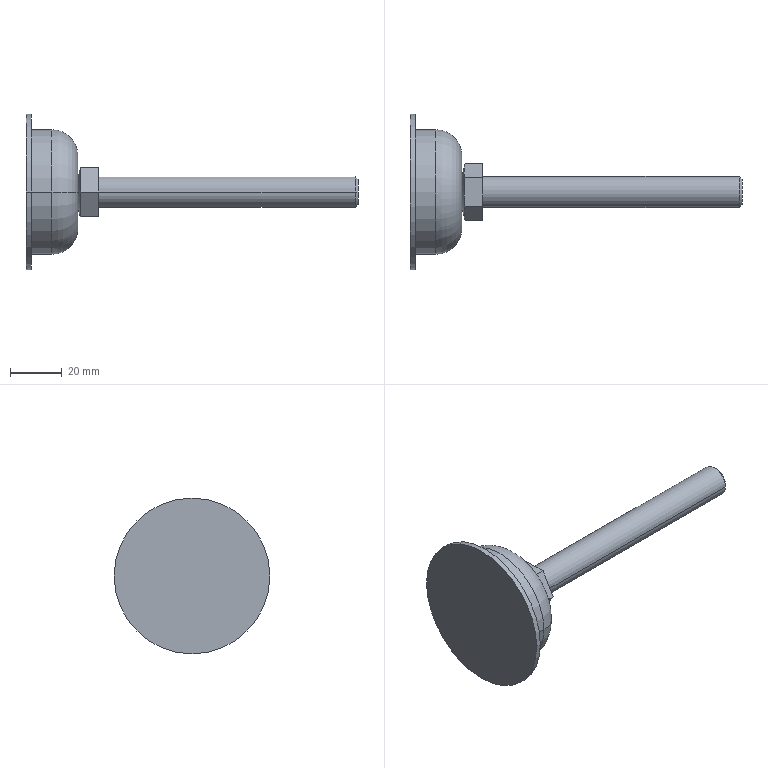Part | SolidWorks | features RefAxis 9, 3DProfileFeature 3, ICE 1, Revolution 1 | 1 solid | 23 faces | box 128 x 60 x 60 mm | volume 48974 mm3 | plane 11 | cylinder 6 | cone 4 | torus 2 | commonest cylinder face diameters 12 x2 48 x2 60 x2
STEP:
#1=CARTESIAN_POINT('',(28.,6.,0.));
#2=VERTEX_POINT('',#1);
#3=CARTESIAN_POINT('',(28.,-6.,0.));
#4=VERTEX_POINT('',#3);
#5=CARTESIAN_POINT('',(28.,0.,0.));
#6=DIRECTION('',(1.,0.,0.));
#7=DIRECTION('',(0.,1.,0.));
#8=AXIS2_PLACEMENT_3D('',#5,#6,#7);
#9=CIRCLE('',#8,6.);
#10=EDGE_CURVE('',#2,#4,#9,.T.);
#11=ORIENTED_EDGE('',*,*,#10,.T.);
#12=CARTESIAN_POINT('',(126.927,-6.,0.));
#13=VERTEX_POINT('',#12);
#14=CARTESIAN_POINT('',(0.,-6.,0.));
#15=DIRECTION('',(1.,0.,0.));
#16=VECTOR('',#15,1000.);
#17=LINE('',#14,#16);
#18=EDGE_CURVE('',#4,#13,#17,.T.);
#19=ORIENTED_EDGE('',*,*,#18,.T.);
#20=CARTESIAN_POINT('',(126.927,6.,0.));
#21=VERTEX_POINT('',#20);
#22=CARTESIAN_POINT('',(126.927,0.,0.));
#23=DIRECTION('',(1.,0.,0.));
#24=DIRECTION('',(0.,1.,0.));
#25=AXIS2_PLACEMENT_3D('',#22,#23,#24);
#26=CIRCLE('',#25,6.);
#27=EDGE_CURVE('',#21,#13,#26,.T.);
#28=ORIENTED_EDGE('',*,*,#27,.F.);
#29=CARTESIAN_POINT('',(0.,6.,0.));
#30=DIRECTION('',(1.,0.,0.));
#31=VECTOR('',#30,1000.);
#32=LINE('',#29,#31);
#33=EDGE_CURVE('',#2,#21,#32,.T.);
#34=ORIENTED_EDGE('',*,*,#33,.F.);
#35=EDGE_LOOP('',(#11,#19,#28,#34));
#36=FACE_OUTER_BOUND('',#35,.T.);
#37=CARTESIAN_POINT('',(0.,0.,0.));
#38=DIRECTION('',(1.,0.,0.));
#39=DIRECTION('',(0.,1.,0.));
#40=AXIS2_PLACEMENT_3D('',#37,#38,#39);
#41=CYLINDRICAL_SURFACE('',#40,6.);
#42=ADVANCED_FACE('',(#36),#41,.T.);
#43=CARTESIAN_POINT('',(128.,4.927,0.));
#44=VERTEX_POINT('',#43);
#45=CARTESIAN_POINT('',(128.,-4.926,0.));
#46=VERTEX_POINT('',#45);
#47=CARTESIAN_POINT('',(128.,0.,0.));
#48=DIRECTION('',(1.,0.,0.));
#49=DIRECTION('',(0.,1.,0.));
#50=AXIS2_PLACEMENT_3D('',#47,#48,#49);
#51=CIRCLE('',#50,4.926);
#52=EDGE_CURVE('',#44,#46,#51,.T.);
#53=ORIENTED_EDGE('',*,*,#52,.F.);
#54=CARTESIAN_POINT('',(126.927,6.,0.));
#55=DIRECTION('',(-0.7071,0.7071,0.));
#56=VECTOR('',#55,1000.);
#57=LINE('',#54,#56);
#58=EDGE_CURVE('',#44,#21,#57,.T.);
#59=ORIENTED_EDGE('',*,*,#58,.T.);
#60=ORIENTED_EDGE('',*,*,#27,.T.);
#61=CARTESIAN_POINT('',(126.927,-6.,0.));
#62=DIRECTION('',(-0.7071,-0.7071,0.));
#63=VECTOR('',#62,1000.);
#64=LINE('',#61,#63);
#65=EDGE_CURVE('',#46,#13,#64,.T.);
#66=ORIENTED_EDGE('',*,*,#65,.F.);
#67=EDGE_LOOP('',(#53,#59,#60,#66));
#68=FACE_OUTER_BOUND('',#67,.T.);
#69=CARTESIAN_POINT('',(126.927,0.,0.));
#70=DIRECTION('',(-1.,0.,0.));
#71=DIRECTION('',(0.,-1.,0.));
#72=AXIS2_PLACEMENT_3D('',#69,#70,#71);
#73=CONICAL_SURFACE('',#72,6.,0.7854);
#74=ADVANCED_FACE('',(#68),#73,.T.);
#75=CARTESIAN_POINT('',(0.,30.,0.));
#76=VERTEX_POINT('',#75);
#77=CARTESIAN_POINT('',(0.,-30.,0.));
#78=VERTEX_POINT('',#77);
#79=CARTESIAN_POINT('',(0.,0.,0.));
#80=DIRECTION('',(1.,0.,0.));
#81=DIRECTION('',(0.,1.,0.));
#82=AXIS2_PLACEMENT_3D('',#79,#80,#81);
#83=CIRCLE('',#82,30.);
#84=EDGE_CURVE('',#76,#78,#83,.T.);
#85=ORIENTED_EDGE('',*,*,#84,.T.);
#86=CARTESIAN_POINT('',(2.,-30.,0.));
#87=VERTEX_POINT('',#86);
#88=CARTESIAN_POINT('',(0.,-30.,0.));
#89=DIRECTION('',(1.,0.,0.));
#90=VECTOR('',#89,1000.);
#91=LINE('',#88,#90);
#92=EDGE_CURVE('',#78,#87,#91,.T.);
#93=ORIENTED_EDGE('',*,*,#92,.T.);
#94=CARTESIAN_POINT('',(2.,30.,0.));
#95=VERTEX_POINT('',#94);
#96=CARTESIAN_POINT('',(2.,0.,0.));
#97=DIRECTION('',(1.,0.,0.));
#98=DIRECTION('',(0.,1.,0.));
#99=AXIS2_PLACEMENT_3D('',#96,#97,#98);
#100=CIRCLE('',#99,30.);
#101=EDGE_CURVE('',#95,#87,#100,.T.);
#102=ORIENTED_EDGE('',*,*,#101,.F.);
#103=CARTESIAN_POINT('',(0.,30.,0.));
#104=DIRECTION('',(1.,0.,0.));
#105=VECTOR('',#104,1000.);
#106=LINE('',#103,#105);
#107=EDGE_CURVE('',#76,#95,#106,.T.);
#108=ORIENTED_EDGE('',*,*,#107,.F.);
#109=EDGE_LOOP('',(#85,#93,#102,#108));
#110=FACE_OUTER_BOUND('',#109,.T.);
#111=CARTESIAN_POINT('',(0.,0.,0.));
#112=DIRECTION('',(1.,0.,0.));
#113=DIRECTION('',(0.,1.,0.));
#114=AXIS2_PLACEMENT_3D('',#111,#112,#113);
#115=CYLINDRICAL_SURFACE('',#114,30.);
#116=ADVANCED_FACE('',(#110),#115,.T.);
#117=CARTESIAN_POINT('',(2.,24.,0.));
#118=VERTEX_POINT('',#117);
#119=CARTESIAN_POINT('',(2.,-24.,0.));
#120=VERTEX_POINT('',#119);
#121=CARTESIAN_POINT('',(2.,0.,0.));
#122=DIRECTION('',(1.,0.,0.));
#123=DIRECTION('',(0.,1.,0.));
#124=AXIS2_PLACEMENT_3D('',#121,#122,#123);
#125=CIRCLE('',#124,24.);
#126=EDGE_CURVE('',#118,#120,#125,.T.);
#127=ORIENTED_EDGE('',*,*,#126,.T.);
#128=CARTESIAN_POINT('',(10.,-24.,0.));
#129=VERTEX_POINT('',#128);
#130=CARTESIAN_POINT('',(0.,-24.,0.));
#131=DIRECTION('',(1.,0.,0.));
#132=VECTOR('',#131,1000.);
#133=LINE('',#130,#132);
#134=EDGE_CURVE('',#120,#129,#133,.T.);
#135=ORIENTED_EDGE('',*,*,#134,.T.);
#136=CARTESIAN_POINT('',(10.,24.,0.));
#137=VERTEX_POINT('',#136);
#138=CARTESIAN_POINT('',(10.,0.,0.));
#139=DIRECTION('',(1.,0.,0.));
#140=DIRECTION('',(0.,1.,0.));
#141=AXIS2_PLACEMENT_3D('',#138,#139,#140);
#142=CIRCLE('',#141,24.);
#143=EDGE_CURVE('',#137,#129,#142,.T.);
#144=ORIENTED_EDGE('',*,*,#143,.F.);
#145=CARTESIAN_POINT('',(0.,24.,0.));
#146=DIRECTION('',(1.,0.,0.));
#147=VECTOR('',#146,1000.);
#148=LINE('',#145,#147);
#149=EDGE_CURVE('',#118,#137,#148,.T.);
#150=ORIENTED_EDGE('',*,*,#149,.F.);
#151=EDGE_LOOP('',(#127,#135,#144,#150));
#152=FACE_OUTER_BOUND('',#151,.T.);
#153=CARTESIAN_POINT('',(0.,0.,0.));
#154=DIRECTION('',(1.,0.,0.));
#155=DIRECTION('',(0.,1.,0.));
#156=AXIS2_PLACEMENT_3D('',#153,#154,#155);
#157=CYLINDRICAL_SURFACE('',#156,24.);
#158=ADVANCED_FACE('',(#152),#157,.T.);
#159=ORIENTED_EDGE('',*,*,#143,.T.);
#160=CARTESIAN_POINT('',(20.,-14.,0.));
#161=VERTEX_POINT('',#160);
#162=CARTESIAN_POINT('',(10.,-14.,0.));
#163=DIRECTION('',(0.,0.,1.));
#164=DIRECTION('',(0.,-1.,0.));
#165=AXIS2_PLACEMENT_3D('',#162,#163,#164);
#166=CIRCLE('',#165,10.);
#167=EDGE_CURVE('',#129,#161,#166,.T.);
#168=ORIENTED_EDGE('',*,*,#167,.T.);
#169=CARTESIAN_POINT('',(20.,14.,0.));
#170=VERTEX_POINT('',#169);
#171=CARTESIAN_POINT('',(20.,0.,0.));
#172=DIRECTION('',(1.,0.,0.));
#173=DIRECTION('',(0.,1.,0.));
#174=AXIS2_PLACEMENT_3D('',#171,#172,#173);
#175=CIRCLE('',#174,14.);
#176=EDGE_CURVE('',#170,#161,#175,.T.);
#177=ORIENTED_EDGE('',*,*,#176,.F.);
#178=CARTESIAN_POINT('',(10.,14.,0.));
#179=DIRECTION('',(0.,0.,-1.));
#180=DIRECTION('',(-1.,0.,0.));
#181=AXIS2_PLACEMENT_3D('',#178,#179,#180);
#182=CIRCLE('',#181,10.);
#183=EDGE_CURVE('',#137,#170,#182,.T.);
#184=ORIENTED_EDGE('',*,*,#183,.F.);
#185=EDGE_LOOP('',(#159,#168,#177,#184));
#186=FACE_OUTER_BOUND('',#185,.T.);
#187=CARTESIAN_POINT('',(10.,0.,0.));
#188=DIRECTION('',(1.,0.,0.));
#189=DIRECTION('',(0.,1.,0.));
#190=AXIS2_PLACEMENT_3D('',#187,#188,#189);
#191=TOROIDAL_SURFACE('',#190,14.,10.);
#192=ADVANCED_FACE('',(#186),#191,.T.);
#193=CARTESIAN_POINT('',(20.,6.,0.));
#194=VERTEX_POINT('',#193);
#195=CARTESIAN_POINT('',(20.,-6.,0.));
#196=VERTEX_POINT('',#195);
#197=CARTESIAN_POINT('',(20.,0.,0.));
#198=DIRECTION('',(1.,0.,0.));
#199=DIRECTION('',(0.,1.,0.));
#200=AXIS2_PLACEMENT_3D('',#197,#198,#199);
#201=CIRCLE('',#200,6.);
#202=EDGE_CURVE('',#194,#196,#201,.T.);
#203=ORIENTED_EDGE('',*,*,#202,.T.);
#204=CARTESIAN_POINT('',(21.236,-10.97,0.));
#205=VERTEX_POINT('',#204);
#206=CARTESIAN_POINT('',(20.,-6.,0.));
#207=DIRECTION('',(0.2414,-0.9704,0.));
#208=VECTOR('',#207,1000.);
#209=LINE('',#206,#208);
#210=EDGE_CURVE('',#196,#205,#209,.T.);
#211=ORIENTED_EDGE('',*,*,#210,.T.);
#212=CARTESIAN_POINT('',(21.236,-5.485,9.5));
#213=VERTEX_POINT('',#212);
#214=CARTESIAN_POINT('',(21.236,-5.485,9.5));
#215=CARTESIAN_POINT('',(21.123,-5.942,8.708));
#216=CARTESIAN_POINT('',(21.03,-6.399,7.917));
#217=CARTESIAN_POINT('',(20.904,-7.313,6.333));
#218=CARTESIAN_POINT('',(20.837,-8.227,4.75));
#219=CARTESIAN_POINT('',(20.904,-9.141,3.167));
#220=CARTESIAN_POINT('',(21.03,-10.056,1.583));
#221=CARTESIAN_POINT('',(21.123,-10.513,0.7917));
#222=CARTESIAN_POINT('',(21.236,-10.97,0.));
#223=B_SPLINE_CURVE_WITH_KNOTS('',3,(#214,#215,#216,#217,#218,#219,#220,#221,#222),.UNSPECIFIED.,.F.,.F.,(4,2,1,2,4),(0.000000231,0.002743,0.005485,0.008227,0.01097),.UNSPECIFIED.);
#224=EDGE_CURVE('',#213,#205,#223,.T.);
#225=ORIENTED_EDGE('',*,*,#224,.F.);
#226=CARTESIAN_POINT('',(21.236,5.485,9.5));
#227=VERTEX_POINT('',#226);
#228=CARTESIAN_POINT('',(21.236,5.485,9.5));
#229=CARTESIAN_POINT('',(21.01,3.662,9.5));
#230=CARTESIAN_POINT('',(20.871,1.837,9.5));
#231=CARTESIAN_POINT('',(20.871,-0.9062,9.5));
#232=CARTESIAN_POINT('',(20.904,-1.822,9.5));
#233=CARTESIAN_POINT('',(21.03,-3.654,9.5));
#234=CARTESIAN_POINT('',(21.123,-4.572,9.5));
#235=CARTESIAN_POINT('',(21.236,-5.485,9.5));
#236=B_SPLINE_CURVE_WITH_KNOTS('',3,(#228,#229,#230,#231,#232,#233,#234,#235),.UNSPECIFIED.,.F.,.F.,(4,2,2,4),(0.02128,0.02679,0.02955,0.0323),.UNSPECIFIED.);
#237=EDGE_CURVE('',#227,#213,#236,.T.);
#238=ORIENTED_EDGE('',*,*,#237,.F.);
#239=CARTESIAN_POINT('',(21.236,10.97,0.));
#240=VERTEX_POINT('',#239);
#241=CARTESIAN_POINT('',(21.236,10.97,0.));
#242=CARTESIAN_POINT('',(21.123,10.513,0.7917));
#243=CARTESIAN_POINT('',(21.03,10.056,1.583));
#244=CARTESIAN_POINT('',(20.904,9.141,3.167));
#245=CARTESIAN_POINT('',(20.837,8.227,4.75));
#246=CARTESIAN_POINT('',(20.904,7.313,6.333));
#247=CARTESIAN_POINT('',(21.03,6.399,7.917));
#248=CARTESIAN_POINT('',(21.123,5.942,8.708));
#249=CARTESIAN_POINT('',(21.236,5.485,9.5));
#250=B_SPLINE_CURVE_WITH_KNOTS('',3,(#241,#242,#243,#244,#245,#246,#247,#248,#249),.UNSPECIFIED.,.F.,.F.,(4,2,1,2,4),(0.000000231,0.002743,0.005485,0.008227,0.01097),.UNSPECIFIED.);
#251=EDGE_CURVE('',#240,#227,#250,.T.);
#252=ORIENTED_EDGE('',*,*,#251,.F.);
#253=CARTESIAN_POINT('',(20.,6.,0.));
#254=DIRECTION('',(0.2414,0.9704,0.));
#255=VECTOR('',#254,1000.);
#256=LINE('',#253,#255);
#257=EDGE_CURVE('',#194,#240,#256,.T.);
#258=ORIENTED_EDGE('',*,*,#257,.F.);
#259=EDGE_LOOP('',(#203,#211,#225,#238,#252,#258));
#260=FACE_OUTER_BOUND('',#259,.T.);
#261=CARTESIAN_POINT('',(20.,0.,0.));
#262=DIRECTION('',(1.,0.,0.));
#263=DIRECTION('',(0.,1.,0.));
#264=AXIS2_PLACEMENT_3D('',#261,#262,#263);
#265=CONICAL_SURFACE('',#264,6.,1.327);
#266=ADVANCED_FACE('',(#260),#265,.T.);
#267=ORIENTED_EDGE('',*,*,#210,.F.);
#268=CARTESIAN_POINT('',(20.,0.,0.));
#269=DIRECTION('',(1.,0.,0.));
#270=DIRECTION('',(0.,1.,0.));
#271=AXIS2_PLACEMENT_3D('',#268,#269,#270);
#272=CIRCLE('',#271,6.);
#273=EDGE_CURVE('',#196,#194,#272,.T.);
#274=ORIENTED_EDGE('',*,*,#273,.T.);
#275=ORIENTED_EDGE('',*,*,#257,.T.);
#276=CARTESIAN_POINT('',(21.236,5.485,-9.5));
#277=VERTEX_POINT('',#276);
#278=CARTESIAN_POINT('',(21.236,5.485,-9.5));
#279=CARTESIAN_POINT('',(21.123,5.942,-8.708));
#280=CARTESIAN_POINT('',(21.03,6.399,-7.917));
#281=CARTESIAN_POINT('',(20.904,7.313,-6.333));
#282=CARTESIAN_POINT('',(20.837,8.227,-4.75));
#283=CARTESIAN_POINT('',(20.904,9.141,-3.167));
#284=CARTESIAN_POINT('',(21.03,10.056,-1.583));
#285=CARTESIAN_POINT('',(21.123,10.513,-0.7917));
#286=CARTESIAN_POINT('',(21.236,10.97,0.));
#287=B_SPLINE_CURVE_WITH_KNOTS('',3,(#278,#279,#280,#281,#282,#283,#284,#285,#286),.UNSPECIFIED.,.F.,.F.,(4,2,1,2,4),(0.000000231,0.002743,0.005485,0.008227,0.01097),.UNSPECIFIED.);
#288=EDGE_CURVE('',#277,#240,#287,.T.);
#289=ORIENTED_EDGE('',*,*,#288,.F.);
#290=CARTESIAN_POINT('',(21.236,-5.485,-9.5));
#291=VERTEX_POINT('',#290);
#292=CARTESIAN_POINT('',(21.236,-5.485,-9.5));
#293=CARTESIAN_POINT('',(21.123,-4.572,-9.5));
#294=CARTESIAN_POINT('',(21.03,-3.654,-9.5));
#295=CARTESIAN_POINT('',(20.904,-1.822,-9.5));
#296=CARTESIAN_POINT('',(20.871,-0.9062,-9.5));
#297=CARTESIAN_POINT('',(20.871,1.837,-9.5));
#298=CARTESIAN_POINT('',(21.01,3.662,-9.5));
#299=CARTESIAN_POINT('',(21.236,5.485,-9.5));
#300=B_SPLINE_CURVE_WITH_KNOTS('',3,(#292,#293,#294,#295,#296,#297,#298,#299),.UNSPECIFIED.,.F.,.F.,(4,2,2,4),(0.009106,0.01186,0.01462,0.02014),.UNSPECIFIED.);
#301=EDGE_CURVE('',#291,#277,#300,.T.);
#302=ORIENTED_EDGE('',*,*,#301,.F.);
#303=CARTESIAN_POINT('',(21.236,-10.97,0.));
#304=CARTESIAN_POINT('',(21.123,-10.513,-0.7917));
#305=CARTESIAN_POINT('',(21.03,-10.056,-1.583));
#306=CARTESIAN_POINT('',(20.904,-9.141,-3.167));
#307=CARTESIAN_POINT('',(20.837,-8.227,-4.75));
#308=CARTESIAN_POINT('',(20.904,-7.313,-6.333));
#309=CARTESIAN_POINT('',(21.03,-6.399,-7.917));
#310=CARTESIAN_POINT('',(21.123,-5.942,-8.708));
#311=CARTESIAN_POINT('',(21.236,-5.485,-9.5));
#312=B_SPLINE_CURVE_WITH_KNOTS('',3,(#303,#304,#305,#306,#307,#308,#309,#310,#311),.UNSPECIFIED.,.F.,.F.,(4,2,1,2,4),(0.000000231,0.002743,0.005485,0.008227,0.01097),.UNSPECIFIED.);
#313=EDGE_CURVE('',#205,#291,#312,.T.);
#314=ORIENTED_EDGE('',*,*,#313,.F.);
#315=EDGE_LOOP('',(#267,#274,#275,#289,#302,#314));
#316=FACE_OUTER_BOUND('',#315,.T.);
#317=CARTESIAN_POINT('',(20.,0.,0.));
#318=DIRECTION('',(1.,0.,0.));
#319=DIRECTION('',(0.,1.,0.));
#320=AXIS2_PLACEMENT_3D('',#317,#318,#319);
#321=CONICAL_SURFACE('',#320,6.,1.327);
#322=ADVANCED_FACE('',(#316),#321,.T.);
#323=ORIENTED_EDGE('',*,*,#176,.T.);
#324=CARTESIAN_POINT('',(20.,0.,0.));
#325=DIRECTION('',(1.,0.,0.));
#326=DIRECTION('',(0.,1.,0.));
#327=AXIS2_PLACEMENT_3D('',#324,#325,#326);
#328=CIRCLE('',#327,14.);
#329=EDGE_CURVE('',#161,#170,#328,.T.);
#330=ORIENTED_EDGE('',*,*,#329,.T.);
#331=EDGE_LOOP('',(#323,#330));
#332=FACE_OUTER_BOUND('',#331,.T.);
#333=ORIENTED_EDGE('',*,*,#202,.F.);
#334=ORIENTED_EDGE('',*,*,#273,.F.);
#335=EDGE_LOOP('',(#333,#334));
#336=FACE_BOUND('',#335,.T.);
#337=CARTESIAN_POINT('',(20.,-6.,0.));
#338=DIRECTION('',(-1.,0.,0.));
#339=DIRECTION('',(0.,-1.,0.));
#340=AXIS2_PLACEMENT_3D('',#337,#338,#339);
#341=PLANE('',#340);
#342=ADVANCED_FACE('',(#332,#336),#341,.F.);
#343=ORIENTED_EDGE('',*,*,#167,.F.);
#344=CARTESIAN_POINT('',(10.,0.,0.));
#345=DIRECTION('',(1.,0.,0.));
#346=DIRECTION('',(0.,1.,0.));
#347=AXIS2_PLACEMENT_3D('',#344,#345,#346);
#348=CIRCLE('',#347,24.);
#349=EDGE_CURVE('',#129,#137,#348,.T.);
#350=ORIENTED_EDGE('',*,*,#349,.T.);
#351=ORIENTED_EDGE('',*,*,#183,.T.);
#352=ORIENTED_EDGE('',*,*,#329,.F.);
#353=EDGE_LOOP('',(#343,#350,#351,#352));
#354=FACE_OUTER_BOUND('',#353,.T.);
#355=CARTESIAN_POINT('',(10.,0.,0.));
#356=DIRECTION('',(1.,0.,0.));
#357=DIRECTION('',(0.,1.,0.));
#358=AXIS2_PLACEMENT_3D('',#355,#356,#357);
#359=TOROIDAL_SURFACE('',#358,14.,10.);
#360=ADVANCED_FACE('',(#354),#359,.T.);
#361=ORIENTED_EDGE('',*,*,#134,.F.);
#362=CARTESIAN_POINT('',(2.,0.,0.));
#363=DIRECTION('',(1.,0.,0.));
#364=DIRECTION('',(0.,1.,0.));
#365=AXIS2_PLACEMENT_3D('',#362,#363,#364);
#366=CIRCLE('',#365,24.);
#367=EDGE_CURVE('',#120,#118,#366,.T.);
#368=ORIENTED_EDGE('',*,*,#367,.T.);
#369=ORIENTED_EDGE('',*,*,#149,.T.);
#370=ORIENTED_EDGE('',*,*,#349,.F.);
#371=EDGE_LOOP('',(#361,#368,#369,#370));
#372=FACE_OUTER_BOUND('',#371,.T.);
#373=CARTESIAN_POINT('',(0.,0.,0.));
#374=DIRECTION('',(1.,0.,0.));
#375=DIRECTION('',(0.,1.,0.));
#376=AXIS2_PLACEMENT_3D('',#373,#374,#375);
#377=CYLINDRICAL_SURFACE('',#376,24.);
#378=ADVANCED_FACE('',(#372),#377,.T.);
#379=ORIENTED_EDGE('',*,*,#126,.F.);
#380=ORIENTED_EDGE('',*,*,#367,.F.);
#381=EDGE_LOOP('',(#379,#380));
#382=FACE_BOUND('',#381,.T.);
#383=ORIENTED_EDGE('',*,*,#101,.T.);
#384=CARTESIAN_POINT('',(2.,0.,0.));
#385=DIRECTION('',(1.,0.,0.));
#386=DIRECTION('',(0.,1.,0.));
#387=AXIS2_PLACEMENT_3D('',#384,#385,#386);
#388=CIRCLE('',#387,30.);
#389=EDGE_CURVE('',#87,#95,#388,.T.);
#390=ORIENTED_EDGE('',*,*,#389,.T.);
#391=EDGE_LOOP('',(#383,#390));
#392=FACE_OUTER_BOUND('',#391,.T.);
#393=CARTESIAN_POINT('',(2.,-24.,0.));
#394=DIRECTION('',(-1.,0.,0.));
#395=DIRECTION('',(0.,-1.,0.));
#396=AXIS2_PLACEMENT_3D('',#393,#394,#395);
#397=PLANE('',#396);
#398=ADVANCED_FACE('',(#382,#392),#397,.F.);
#399=ORIENTED_EDGE('',*,*,#92,.F.);
#400=CARTESIAN_POINT('',(0.,0.,0.));
#401=DIRECTION('',(1.,0.,0.));
#402=DIRECTION('',(0.,1.,0.));
#403=AXIS2_PLACEMENT_3D('',#400,#401,#402);
#404=CIRCLE('',#403,30.);
#405=EDGE_CURVE('',#78,#76,#404,.T.);
#406=ORIENTED_EDGE('',*,*,#405,.T.);
#407=ORIENTED_EDGE('',*,*,#107,.T.);
#408=ORIENTED_EDGE('',*,*,#389,.F.);
#409=EDGE_LOOP('',(#399,#406,#407,#408));
#410=FACE_OUTER_BOUND('',#409,.T.);
#411=CARTESIAN_POINT('',(0.,0.,0.));
#412=DIRECTION('',(1.,0.,0.));
#413=DIRECTION('',(0.,1.,0.));
#414=AXIS2_PLACEMENT_3D('',#411,#412,#413);
#415=CYLINDRICAL_SURFACE('',#414,30.);
#416=ADVANCED_FACE('',(#410),#415,.T.);
#417=ORIENTED_EDGE('',*,*,#84,.F.);
#418=ORIENTED_EDGE('',*,*,#405,.F.);
#419=EDGE_LOOP('',(#417,#418));
#420=FACE_OUTER_BOUND('',#419,.T.);
#421=CARTESIAN_POINT('',(0.,-30.,0.));
#422=DIRECTION('',(1.,0.,0.));
#423=DIRECTION('',(0.,1.,0.));
#424=AXIS2_PLACEMENT_3D('',#421,#422,#423);
#425=PLANE('',#424);
#426=ADVANCED_FACE('',(#420),#425,.F.);
#427=ORIENTED_EDGE('',*,*,#251,.T.);
#428=CARTESIAN_POINT('',(28.,5.485,9.5));
#429=VERTEX_POINT('',#428);
#430=CARTESIAN_POINT('',(20.,5.485,9.5));
#431=DIRECTION('',(1.,0.,0.));
#432=VECTOR('',#431,1000.);
#433=LINE('',#430,#432);
#434=EDGE_CURVE('',#227,#429,#433,.T.);
#435=ORIENTED_EDGE('',*,*,#434,.T.);
#436=CARTESIAN_POINT('',(28.,10.97,0.));
#437=VERTEX_POINT('',#436);
#438=CARTESIAN_POINT('',(28.,10.97,0.));
#439=DIRECTION('',(0.,-0.5,0.866));
#440=VECTOR('',#439,1000.);
#441=LINE('',#438,#440);
#442=EDGE_CURVE('',#437,#429,#441,.T.);
#443=ORIENTED_EDGE('',*,*,#442,.F.);
#444=CARTESIAN_POINT('',(20.,10.97,0.));
#445=DIRECTION('',(1.,0.,0.));
#446=VECTOR('',#445,1000.);
#447=LINE('',#444,#446);
#448=EDGE_CURVE('',#240,#437,#447,.T.);
#449=ORIENTED_EDGE('',*,*,#448,.F.);
#450=EDGE_LOOP('',(#427,#435,#443,#449));
#451=FACE_OUTER_BOUND('',#450,.T.);
#452=CARTESIAN_POINT('',(20.,10.97,0.));
#453=DIRECTION('',(0.,0.866,0.5));
#454=DIRECTION('',(0.,-0.5,0.866));
#455=AXIS2_PLACEMENT_3D('',#452,#453,#454);
#456=PLANE('',#455);
#457=ADVANCED_FACE('',(#451),#456,.T.);
#458=ORIENTED_EDGE('',*,*,#288,.T.);
#459=ORIENTED_EDGE('',*,*,#448,.T.);
#460=CARTESIAN_POINT('',(28.,5.485,-9.5));
#461=VERTEX_POINT('',#460);
#462=CARTESIAN_POINT('',(28.,5.485,-9.5));
#463=DIRECTION('',(0.,0.5,0.866));
#464=VECTOR('',#463,1000.);
#465=LINE('',#462,#464);
#466=EDGE_CURVE('',#461,#437,#465,.T.);
#467=ORIENTED_EDGE('',*,*,#466,.F.);
#468=CARTESIAN_POINT('',(20.,5.485,-9.5));
#469=DIRECTION('',(1.,0.,0.));
#470=VECTOR('',#469,1000.);
#471=LINE('',#468,#470);
#472=EDGE_CURVE('',#277,#461,#471,.T.);
#473=ORIENTED_EDGE('',*,*,#472,.F.);
#474=EDGE_LOOP('',(#458,#459,#467,#473));
#475=FACE_OUTER_BOUND('',#474,.T.);
#476=CARTESIAN_POINT('',(20.,5.485,-9.5));
#477=DIRECTION('',(0.,0.866,-0.5));
#478=DIRECTION('',(0.,0.5,0.866));
#479=AXIS2_PLACEMENT_3D('',#476,#477,#478);
#480=PLANE('',#479);
#481=ADVANCED_FACE('',(#475),#480,.T.);
#482=ORIENTED_EDGE('',*,*,#301,.T.);
#483=ORIENTED_EDGE('',*,*,#472,.T.);
#484=CARTESIAN_POINT('',(28.,-5.485,-9.5));
#485=VERTEX_POINT('',#484);
#486=CARTESIAN_POINT('',(28.,-5.485,-9.5));
#487=DIRECTION('',(0.,1.,0.));
#488=VECTOR('',#487,1000.);
#489=LINE('',#486,#488);
#490=EDGE_CURVE('',#485,#461,#489,.T.);
#491=ORIENTED_EDGE('',*,*,#490,.F.);
#492=CARTESIAN_POINT('',(20.,-5.485,-9.5));
#493=DIRECTION('',(1.,0.,0.));
#494=VECTOR('',#493,1000.);
#495=LINE('',#492,#494);
#496=EDGE_CURVE('',#291,#485,#495,.T.);
#497=ORIENTED_EDGE('',*,*,#496,.F.);
#498=EDGE_LOOP('',(#482,#483,#491,#497));
#499=FACE_OUTER_BOUND('',#498,.T.);
#500=CARTESIAN_POINT('',(20.,-5.485,-9.5));
#501=DIRECTION('',(0.,0.,-1.));
#502=DIRECTION('',(-1.,0.,0.));
#503=AXIS2_PLACEMENT_3D('',#500,#501,#502);
#504=PLANE('',#503);
#505=ADVANCED_FACE('',(#499),#504,.T.);
#506=ORIENTED_EDGE('',*,*,#313,.T.);
#507=ORIENTED_EDGE('',*,*,#496,.T.);
#508=CARTESIAN_POINT('',(28.,-10.97,0.));
#509=VERTEX_POINT('',#508);
#510=CARTESIAN_POINT('',(28.,-10.97,0.));
#511=DIRECTION('',(0.,0.5,-0.866));
#512=VECTOR('',#511,1000.);
#513=LINE('',#510,#512);
#514=EDGE_CURVE('',#509,#485,#513,.T.);
#515=ORIENTED_EDGE('',*,*,#514,.F.);
#516=CARTESIAN_POINT('',(20.,-10.97,0.));
#517=DIRECTION('',(1.,0.,0.));
#518=VECTOR('',#517,1000.);
#519=LINE('',#516,#518);
#520=EDGE_CURVE('',#205,#509,#519,.T.);
#521=ORIENTED_EDGE('',*,*,#520,.F.);
#522=EDGE_LOOP('',(#506,#507,#515,#521));
#523=FACE_OUTER_BOUND('',#522,.T.);
#524=CARTESIAN_POINT('',(20.,-10.97,0.));
#525=DIRECTION('',(0.,-0.866,-0.5));
#526=DIRECTION('',(0.,0.5,-0.866));
#527=AXIS2_PLACEMENT_3D('',#524,#525,#526);
#528=PLANE('',#527);
#529=ADVANCED_FACE('',(#523),#528,.T.);
#530=ORIENTED_EDGE('',*,*,#224,.T.);
#531=ORIENTED_EDGE('',*,*,#520,.T.);
#532=CARTESIAN_POINT('',(28.,-5.485,9.5));
#533=VERTEX_POINT('',#532);
#534=CARTESIAN_POINT('',(28.,-5.485,9.5));
#535=DIRECTION('',(0.,-0.5,-0.866));
#536=VECTOR('',#535,1000.);
#537=LINE('',#534,#536);
#538=EDGE_CURVE('',#533,#509,#537,.T.);
#539=ORIENTED_EDGE('',*,*,#538,.F.);
#540=CARTESIAN_POINT('',(20.,-5.485,9.5));
#541=DIRECTION('',(1.,0.,0.));
#542=VECTOR('',#541,1000.);
#543=LINE('',#540,#542);
#544=EDGE_CURVE('',#213,#533,#543,.T.);
#545=ORIENTED_EDGE('',*,*,#544,.F.);
#546=EDGE_LOOP('',(#530,#531,#539,#545));
#547=FACE_OUTER_BOUND('',#546,.T.);
#548=CARTESIAN_POINT('',(20.,-5.485,9.5));
#549=DIRECTION('',(0.,-0.866,0.5));
#550=DIRECTION('',(0.,-0.5,-0.866));
#551=AXIS2_PLACEMENT_3D('',#548,#549,#550);
#552=PLANE('',#551);
#553=ADVANCED_FACE('',(#547),#552,.T.);
#554=ORIENTED_EDGE('',*,*,#237,.T.);
#555=ORIENTED_EDGE('',*,*,#544,.T.);
#556=CARTESIAN_POINT('',(28.,5.485,9.5));
#557=DIRECTION('',(0.,-1.,0.));
#558=VECTOR('',#557,1000.);
#559=LINE('',#556,#558);
#560=EDGE_CURVE('',#429,#533,#559,.T.);
#561=ORIENTED_EDGE('',*,*,#560,.F.);
#562=ORIENTED_EDGE('',*,*,#434,.F.);
#563=EDGE_LOOP('',(#554,#555,#561,#562));
#564=FACE_OUTER_BOUND('',#563,.T.);
#565=CARTESIAN_POINT('',(20.,5.485,9.5));
#566=DIRECTION('',(0.,0.,1.));
#567=DIRECTION('',(1.,0.,0.));
#568=AXIS2_PLACEMENT_3D('',#565,#566,#567);
#569=PLANE('',#568);
#570=ADVANCED_FACE('',(#564),#569,.T.);
#571=CARTESIAN_POINT('',(128.,0.,0.));
#572=DIRECTION('',(1.,0.,0.));
#573=DIRECTION('',(0.,1.,0.));
#574=AXIS2_PLACEMENT_3D('',#571,#572,#573);
#575=CIRCLE('',#574,4.926);
#576=EDGE_CURVE('',#46,#44,#575,.T.);
#577=ORIENTED_EDGE('',*,*,#576,.T.);
#578=ORIENTED_EDGE('',*,*,#52,.T.);
#579=EDGE_LOOP('',(#577,#578));
#580=FACE_OUTER_BOUND('',#579,.T.);
#581=CARTESIAN_POINT('',(128.,0.,0.));
#582=DIRECTION('',(-1.,0.,0.));
#583=DIRECTION('',(0.,-1.,0.));
#584=AXIS2_PLACEMENT_3D('',#581,#582,#583);
#585=PLANE('',#584);
#586=ADVANCED_FACE('',(#580),#585,.F.);
#587=ORIENTED_EDGE('',*,*,#58,.F.);
#588=ORIENTED_EDGE('',*,*,#576,.F.);
#589=ORIENTED_EDGE('',*,*,#65,.T.);
#590=CARTESIAN_POINT('',(126.927,0.,0.));
#591=DIRECTION('',(1.,0.,0.));
#592=DIRECTION('',(0.,1.,0.));
#593=AXIS2_PLACEMENT_3D('',#590,#591,#592);
#594=CIRCLE('',#593,6.);
#595=EDGE_CURVE('',#13,#21,#594,.T.);
#596=ORIENTED_EDGE('',*,*,#595,.T.);
#597=EDGE_LOOP('',(#587,#588,#589,#596));
#598=FACE_OUTER_BOUND('',#597,.T.);
#599=CARTESIAN_POINT('',(126.927,0.,0.));
#600=DIRECTION('',(-1.,0.,0.));
#601=DIRECTION('',(0.,-1.,0.));
#602=AXIS2_PLACEMENT_3D('',#599,#600,#601);
#603=CONICAL_SURFACE('',#602,6.,0.7854);
#604=ADVANCED_FACE('',(#598),#603,.T.);
#605=ORIENTED_EDGE('',*,*,#18,.F.);
#606=CARTESIAN_POINT('',(28.,0.,0.));
#607=DIRECTION('',(1.,0.,0.));
#608=DIRECTION('',(0.,1.,0.));
#609=AXIS2_PLACEMENT_3D('',#606,#607,#608);
#610=CIRCLE('',#609,6.);
#611=EDGE_CURVE('',#4,#2,#610,.T.);
#612=ORIENTED_EDGE('',*,*,#611,.T.);
#613=ORIENTED_EDGE('',*,*,#33,.T.);
#614=ORIENTED_EDGE('',*,*,#595,.F.);
#615=EDGE_LOOP('',(#605,#612,#613,#614));
#616=FACE_OUTER_BOUND('',#615,.T.);
#617=CARTESIAN_POINT('',(0.,0.,0.));
#618=DIRECTION('',(1.,0.,0.));
#619=DIRECTION('',(0.,1.,0.));
#620=AXIS2_PLACEMENT_3D('',#617,#618,#619);
#621=CYLINDRICAL_SURFACE('',#620,6.);
#622=ADVANCED_FACE('',(#616),#621,.T.);
#623=ORIENTED_EDGE('',*,*,#10,.F.);
#624=ORIENTED_EDGE('',*,*,#611,.F.);
#625=EDGE_LOOP('',(#623,#624));
#626=FACE_BOUND('',#625,.T.);
#627=ORIENTED_EDGE('',*,*,#442,.T.);
#628=ORIENTED_EDGE('',*,*,#560,.T.);
#629=ORIENTED_EDGE('',*,*,#538,.T.);
#630=ORIENTED_EDGE('',*,*,#514,.T.);
#631=ORIENTED_EDGE('',*,*,#490,.T.);
#632=ORIENTED_EDGE('',*,*,#466,.T.);
#633=EDGE_LOOP('',(#627,#628,#629,#630,#631,#632));
#634=FACE_OUTER_BOUND('',#633,.T.);
#635=CARTESIAN_POINT('',(28.,-6.,0.));
#636=DIRECTION('',(-1.,0.,0.));
#637=DIRECTION('',(0.,-1.,0.));
#638=AXIS2_PLACEMENT_3D('',#635,#636,#637);
#639=PLANE('',#638);
#640=ADVANCED_FACE('',(#626,#634),#639,.F.);
#641=CLOSED_SHELL('',(#42,#74,#116,#158,#192,#266,#322,#342,#360,#378,#398,#416,#426,#457,#481,#505,#529,#553,#570,#586,#604,#622,#640));
#642=MANIFOLD_SOLID_BREP('',#641);
#643=CARTESIAN_POINT('',(0.,0.,0.));
#644=DIRECTION('',(0.,0.,1.));
#645=DIRECTION('',(1.,0.,0.));
#646=AXIS2_PLACEMENT_3D('',#643,#644,#645);
#647=(LENGTH_UNIT()NAMED_UNIT(*)SI_UNIT(.MILLI.,.METRE.));
#648=UNCERTAINTY_MEASURE_WITH_UNIT(LENGTH_MEASURE(0.00001),#647,'','');
#649=(NAMED_UNIT(*)PLANE_ANGLE_UNIT()SI_UNIT($,.RADIAN.));
#650=(NAMED_UNIT(*)SI_UNIT($,.STERADIAN.)SOLID_ANGLE_UNIT());
#651=(GEOMETRIC_REPRESENTATION_CONTEXT(3)GLOBAL_UNCERTAINTY_ASSIGNED_CONTEXT((#648))GLOBAL_UNIT_ASSIGNED_CONTEXT((#647,#649,#650))REPRESENTATION_CONTEXT('',''));
#652=ADVANCED_BREP_SHAPE_REPRESENTATION('',(#642,#646),#651);